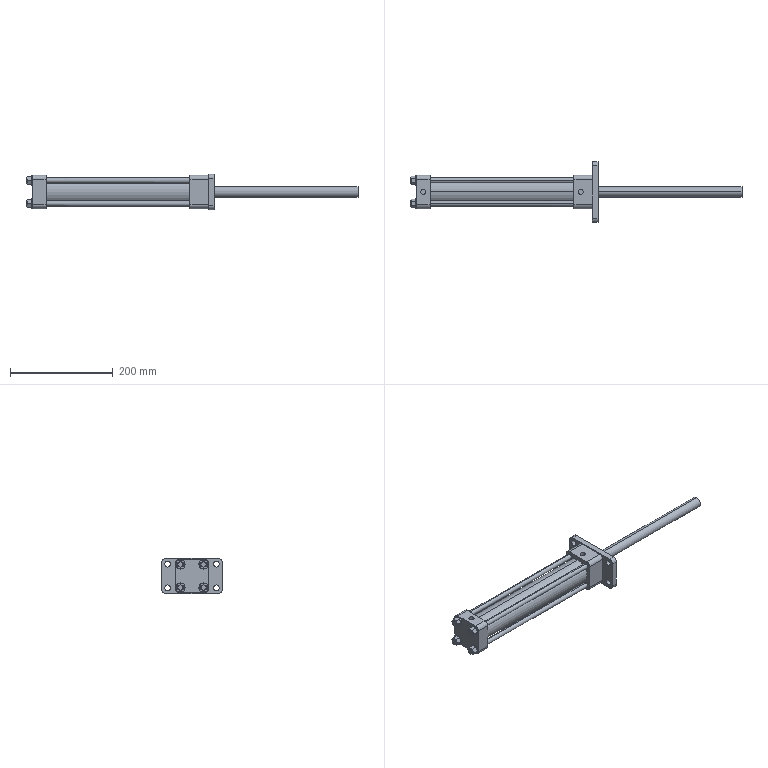Part | Creo | 1 solid | 108 faces | box 646 x 118 x 69 mm | volume 1072698 mm3 | plane 56 | cylinder 52 | commonest cylinder face diameters 10 x20 16 x12 11 x8 18 x8 20 x2 50 x2